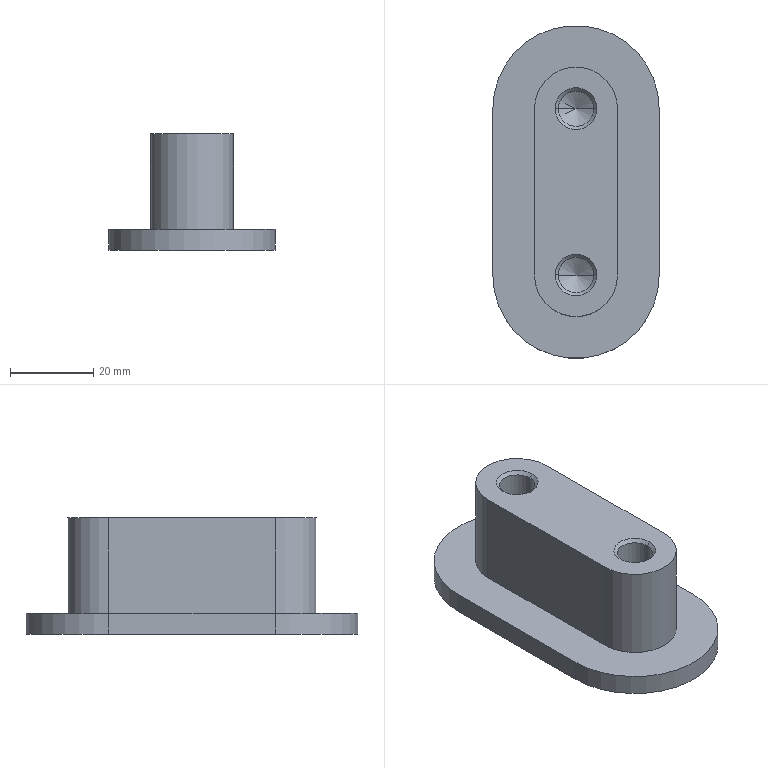Part | SolidWorks | features Extrusion 1, HoleWzd 1, ICE 1 | 1 solid | 23 faces | box 40 x 80 x 28 mm | volume 37305 mm3 | cone 8 | cylinder 8 | plane 7 | commonest cylinder face diameters 8.5 x4 20 x2 40 x2
STEP:
#1=CARTESIAN_POINT('',(-74.25,-60.,27.225));
#2=VERTEX_POINT('',#1);
#3=CARTESIAN_POINT('',(-65.75,-60.,27.225));
#4=VERTEX_POINT('',#3);
#5=CARTESIAN_POINT('',(-70.,-60.,27.225));
#6=DIRECTION('',(0.,0.,1.));
#7=DIRECTION('',(1.,0.,0.));
#8=AXIS2_PLACEMENT_3D('',#5,#6,#7);
#9=CIRCLE('',#8,4.25);
#10=EDGE_CURVE('',#2,#4,#9,.T.);
#11=ORIENTED_EDGE('',*,*,#10,.F.);
#12=CARTESIAN_POINT('',(-75.025,-60.,28.));
#13=VERTEX_POINT('',#12);
#14=CARTESIAN_POINT('',(-75.025,-60.,28.));
#15=DIRECTION('',(-0.7071,0.,0.7071));
#16=VECTOR('',#15,1000.);
#17=LINE('',#14,#16);
#18=EDGE_CURVE('',#2,#13,#17,.T.);
#19=ORIENTED_EDGE('',*,*,#18,.T.);
#20=CARTESIAN_POINT('',(-64.975,-60.,28.));
#21=VERTEX_POINT('',#20);
#22=CARTESIAN_POINT('',(-70.,-60.,28.));
#23=DIRECTION('',(0.,0.,1.));
#24=DIRECTION('',(1.,0.,0.));
#25=AXIS2_PLACEMENT_3D('',#22,#23,#24);
#26=CIRCLE('',#25,5.025);
#27=EDGE_CURVE('',#13,#21,#26,.T.);
#28=ORIENTED_EDGE('',*,*,#27,.T.);
#29=CARTESIAN_POINT('',(-64.975,-60.,28.));
#30=DIRECTION('',(0.7071,0.,0.7071));
#31=VECTOR('',#30,1000.);
#32=LINE('',#29,#31);
#33=EDGE_CURVE('',#4,#21,#32,.T.);
#34=ORIENTED_EDGE('',*,*,#33,.F.);
#35=EDGE_LOOP('',(#11,#19,#28,#34));
#36=FACE_OUTER_BOUND('',#35,.T.);
#37=CARTESIAN_POINT('',(-70.,-60.,28.));
#38=DIRECTION('',(0.,0.,1.));
#39=DIRECTION('',(1.,0.,0.));
#40=AXIS2_PLACEMENT_3D('',#37,#38,#39);
#41=CONICAL_SURFACE('',#40,5.025,0.7854);
#42=ADVANCED_FACE('',(#36),#41,.F.);
#43=CARTESIAN_POINT('',(-74.25,-60.,6.054));
#44=VERTEX_POINT('',#43);
#45=CARTESIAN_POINT('',(-65.75,-60.,6.054));
#46=VERTEX_POINT('',#45);
#47=CARTESIAN_POINT('',(-70.,-60.,6.054));
#48=DIRECTION('',(0.,0.,1.));
#49=DIRECTION('',(1.,0.,0.));
#50=AXIS2_PLACEMENT_3D('',#47,#48,#49);
#51=CIRCLE('',#50,4.25);
#52=EDGE_CURVE('',#44,#46,#51,.T.);
#53=ORIENTED_EDGE('',*,*,#52,.F.);
#54=CARTESIAN_POINT('',(-74.25,-60.,28.));
#55=DIRECTION('',(0.,0.,1.));
#56=VECTOR('',#55,1000.);
#57=LINE('',#54,#56);
#58=EDGE_CURVE('',#44,#2,#57,.T.);
#59=ORIENTED_EDGE('',*,*,#58,.T.);
#60=ORIENTED_EDGE('',*,*,#10,.T.);
#61=CARTESIAN_POINT('',(-65.75,-60.,28.));
#62=DIRECTION('',(0.,0.,1.));
#63=VECTOR('',#62,1000.);
#64=LINE('',#61,#63);
#65=EDGE_CURVE('',#46,#4,#64,.T.);
#66=ORIENTED_EDGE('',*,*,#65,.F.);
#67=EDGE_LOOP('',(#53,#59,#60,#66));
#68=FACE_OUTER_BOUND('',#67,.T.);
#69=CARTESIAN_POINT('',(-70.,-60.,28.));
#70=DIRECTION('',(0.,0.,1.));
#71=DIRECTION('',(1.,0.,0.));
#72=AXIS2_PLACEMENT_3D('',#69,#70,#71);
#73=CYLINDRICAL_SURFACE('',#72,4.25);
#74=ADVANCED_FACE('',(#68),#73,.F.);
#75=CARTESIAN_POINT('',(-70.,-60.,3.5));
#76=VERTEX_POINT('',#75);
#77=CARTESIAN_POINT('',(-65.75,-60.,6.054));
#78=DIRECTION('',(0.8572,0.,0.515));
#79=VECTOR('',#78,1000.);
#80=LINE('',#77,#79);
#81=EDGE_CURVE('',#76,#46,#80,.T.);
#82=ORIENTED_EDGE('',*,*,#81,.F.);
#83=CARTESIAN_POINT('',(-74.25,-60.,6.054));
#84=DIRECTION('',(-0.8572,0.,0.515));
#85=VECTOR('',#84,1000.);
#86=LINE('',#83,#85);
#87=EDGE_CURVE('',#76,#44,#86,.T.);
#88=ORIENTED_EDGE('',*,*,#87,.T.);
#89=ORIENTED_EDGE('',*,*,#52,.T.);
#90=EDGE_LOOP('',(#82,#88,#89));
#91=FACE_OUTER_BOUND('',#90,.T.);
#92=CARTESIAN_POINT('',(-70.,-60.,6.054));
#93=DIRECTION('',(0.,0.,1.));
#94=DIRECTION('',(1.,0.,0.));
#95=AXIS2_PLACEMENT_3D('',#92,#93,#94);
#96=CONICAL_SURFACE('',#95,4.25,1.03);
#97=ADVANCED_FACE('',(#91),#96,.F.);
#98=CARTESIAN_POINT('',(-74.25,-100.,27.225));
#99=VERTEX_POINT('',#98);
#100=CARTESIAN_POINT('',(-65.75,-100.,27.225));
#101=VERTEX_POINT('',#100);
#102=CARTESIAN_POINT('',(-70.,-100.,27.225));
#103=DIRECTION('',(0.,0.,1.));
#104=DIRECTION('',(1.,0.,0.));
#105=AXIS2_PLACEMENT_3D('',#102,#103,#104);
#106=CIRCLE('',#105,4.25);
#107=EDGE_CURVE('',#99,#101,#106,.T.);
#108=ORIENTED_EDGE('',*,*,#107,.F.);
#109=CARTESIAN_POINT('',(-75.025,-100.,28.));
#110=VERTEX_POINT('',#109);
#111=CARTESIAN_POINT('',(-75.025,-100.,28.));
#112=DIRECTION('',(-0.7071,0.,0.7071));
#113=VECTOR('',#112,1000.);
#114=LINE('',#111,#113);
#115=EDGE_CURVE('',#99,#110,#114,.T.);
#116=ORIENTED_EDGE('',*,*,#115,.T.);
#117=CARTESIAN_POINT('',(-64.975,-100.,28.));
#118=VERTEX_POINT('',#117);
#119=CARTESIAN_POINT('',(-70.,-100.,28.));
#120=DIRECTION('',(0.,0.,1.));
#121=DIRECTION('',(1.,0.,0.));
#122=AXIS2_PLACEMENT_3D('',#119,#120,#121);
#123=CIRCLE('',#122,5.025);
#124=EDGE_CURVE('',#110,#118,#123,.T.);
#125=ORIENTED_EDGE('',*,*,#124,.T.);
#126=CARTESIAN_POINT('',(-64.975,-100.,28.));
#127=DIRECTION('',(0.7071,0.,0.7071));
#128=VECTOR('',#127,1000.);
#129=LINE('',#126,#128);
#130=EDGE_CURVE('',#101,#118,#129,.T.);
#131=ORIENTED_EDGE('',*,*,#130,.F.);
#132=EDGE_LOOP('',(#108,#116,#125,#131));
#133=FACE_OUTER_BOUND('',#132,.T.);
#134=CARTESIAN_POINT('',(-70.,-100.,28.));
#135=DIRECTION('',(0.,0.,1.));
#136=DIRECTION('',(1.,0.,0.));
#137=AXIS2_PLACEMENT_3D('',#134,#135,#136);
#138=CONICAL_SURFACE('',#137,5.025,0.7854);
#139=ADVANCED_FACE('',(#133),#138,.F.);
#140=CARTESIAN_POINT('',(-74.25,-100.,6.054));
#141=VERTEX_POINT('',#140);
#142=CARTESIAN_POINT('',(-65.75,-100.,6.054));
#143=VERTEX_POINT('',#142);
#144=CARTESIAN_POINT('',(-70.,-100.,6.054));
#145=DIRECTION('',(0.,0.,1.));
#146=DIRECTION('',(1.,0.,0.));
#147=AXIS2_PLACEMENT_3D('',#144,#145,#146);
#148=CIRCLE('',#147,4.25);
#149=EDGE_CURVE('',#141,#143,#148,.T.);
#150=ORIENTED_EDGE('',*,*,#149,.F.);
#151=CARTESIAN_POINT('',(-74.25,-100.,28.));
#152=DIRECTION('',(0.,0.,1.));
#153=VECTOR('',#152,1000.);
#154=LINE('',#151,#153);
#155=EDGE_CURVE('',#141,#99,#154,.T.);
#156=ORIENTED_EDGE('',*,*,#155,.T.);
#157=ORIENTED_EDGE('',*,*,#107,.T.);
#158=CARTESIAN_POINT('',(-65.75,-100.,28.));
#159=DIRECTION('',(0.,0.,1.));
#160=VECTOR('',#159,1000.);
#161=LINE('',#158,#160);
#162=EDGE_CURVE('',#143,#101,#161,.T.);
#163=ORIENTED_EDGE('',*,*,#162,.F.);
#164=EDGE_LOOP('',(#150,#156,#157,#163));
#165=FACE_OUTER_BOUND('',#164,.T.);
#166=CARTESIAN_POINT('',(-70.,-100.,28.));
#167=DIRECTION('',(0.,0.,1.));
#168=DIRECTION('',(1.,0.,0.));
#169=AXIS2_PLACEMENT_3D('',#166,#167,#168);
#170=CYLINDRICAL_SURFACE('',#169,4.25);
#171=ADVANCED_FACE('',(#165),#170,.F.);
#172=CARTESIAN_POINT('',(-70.,-100.,3.5));
#173=VERTEX_POINT('',#172);
#174=CARTESIAN_POINT('',(-65.75,-100.,6.054));
#175=DIRECTION('',(0.8572,0.,0.515));
#176=VECTOR('',#175,1000.);
#177=LINE('',#174,#176);
#178=EDGE_CURVE('',#173,#143,#177,.T.);
#179=ORIENTED_EDGE('',*,*,#178,.F.);
#180=CARTESIAN_POINT('',(-74.25,-100.,6.054));
#181=DIRECTION('',(-0.8572,0.,0.515));
#182=VECTOR('',#181,1000.);
#183=LINE('',#180,#182);
#184=EDGE_CURVE('',#173,#141,#183,.T.);
#185=ORIENTED_EDGE('',*,*,#184,.T.);
#186=ORIENTED_EDGE('',*,*,#149,.T.);
#187=EDGE_LOOP('',(#179,#185,#186));
#188=FACE_OUTER_BOUND('',#187,.T.);
#189=CARTESIAN_POINT('',(-70.,-100.,6.054));
#190=DIRECTION('',(0.,0.,1.));
#191=DIRECTION('',(1.,0.,0.));
#192=AXIS2_PLACEMENT_3D('',#189,#190,#191);
#193=CONICAL_SURFACE('',#192,4.25,1.03);
#194=ADVANCED_FACE('',(#188),#193,.F.);
#195=CARTESIAN_POINT('',(-60.,-60.,28.));
#196=VERTEX_POINT('',#195);
#197=CARTESIAN_POINT('',(-60.,-60.,5.));
#198=VERTEX_POINT('',#197);
#199=CARTESIAN_POINT('',(-60.,-60.,28.));
#200=DIRECTION('',(0.,0.,-1.));
#201=VECTOR('',#200,1000.);
#202=LINE('',#199,#201);
#203=EDGE_CURVE('',#196,#198,#202,.T.);
#204=ORIENTED_EDGE('',*,*,#203,.T.);
#205=CARTESIAN_POINT('',(-80.,-60.,5.));
#206=VERTEX_POINT('',#205);
#207=CARTESIAN_POINT('',(-70.,-60.,5.));
#208=DIRECTION('',(0.,0.,1.));
#209=DIRECTION('',(1.,0.,0.));
#210=AXIS2_PLACEMENT_3D('',#207,#208,#209);
#211=CIRCLE('',#210,10.);
#212=EDGE_CURVE('',#198,#206,#211,.T.);
#213=ORIENTED_EDGE('',*,*,#212,.T.);
#214=CARTESIAN_POINT('',(-80.,-60.,28.));
#215=VERTEX_POINT('',#214);
#216=CARTESIAN_POINT('',(-80.,-60.,28.));
#217=DIRECTION('',(0.,0.,-1.));
#218=VECTOR('',#217,1000.);
#219=LINE('',#216,#218);
#220=EDGE_CURVE('',#215,#206,#219,.T.);
#221=ORIENTED_EDGE('',*,*,#220,.F.);
#222=CARTESIAN_POINT('',(-70.,-60.,28.));
#223=DIRECTION('',(0.,0.,1.));
#224=DIRECTION('',(1.,0.,0.));
#225=AXIS2_PLACEMENT_3D('',#222,#223,#224);
#226=CIRCLE('',#225,10.);
#227=EDGE_CURVE('',#196,#215,#226,.T.);
#228=ORIENTED_EDGE('',*,*,#227,.F.);
#229=EDGE_LOOP('',(#204,#213,#221,#228));
#230=FACE_OUTER_BOUND('',#229,.T.);
#231=CARTESIAN_POINT('',(-70.,-60.,28.));
#232=DIRECTION('',(0.,0.,-1.));
#233=DIRECTION('',(-1.,0.,0.));
#234=AXIS2_PLACEMENT_3D('',#231,#232,#233);
#235=CYLINDRICAL_SURFACE('',#234,10.);
#236=ADVANCED_FACE('',(#230),#235,.T.);
#237=ORIENTED_EDGE('',*,*,#220,.T.);
#238=CARTESIAN_POINT('',(-80.,-100.,5.));
#239=VERTEX_POINT('',#238);
#240=CARTESIAN_POINT('',(-80.,-60.,5.));
#241=DIRECTION('',(0.,-1.,0.));
#242=VECTOR('',#241,1000.);
#243=LINE('',#240,#242);
#244=EDGE_CURVE('',#206,#239,#243,.T.);
#245=ORIENTED_EDGE('',*,*,#244,.T.);
#246=CARTESIAN_POINT('',(-80.,-100.,28.));
#247=VERTEX_POINT('',#246);
#248=CARTESIAN_POINT('',(-80.,-100.,28.));
#249=DIRECTION('',(0.,0.,-1.));
#250=VECTOR('',#249,1000.);
#251=LINE('',#248,#250);
#252=EDGE_CURVE('',#247,#239,#251,.T.);
#253=ORIENTED_EDGE('',*,*,#252,.F.);
#254=CARTESIAN_POINT('',(-80.,-60.,28.));
#255=DIRECTION('',(0.,-1.,0.));
#256=VECTOR('',#255,1000.);
#257=LINE('',#254,#256);
#258=EDGE_CURVE('',#215,#247,#257,.T.);
#259=ORIENTED_EDGE('',*,*,#258,.F.);
#260=EDGE_LOOP('',(#237,#245,#253,#259));
#261=FACE_OUTER_BOUND('',#260,.T.);
#262=CARTESIAN_POINT('',(-80.,-60.,28.));
#263=DIRECTION('',(1.,0.,0.));
#264=DIRECTION('',(0.,0.,-1.));
#265=AXIS2_PLACEMENT_3D('',#262,#263,#264);
#266=PLANE('',#265);
#267=ADVANCED_FACE('',(#261),#266,.F.);
#268=ORIENTED_EDGE('',*,*,#252,.T.);
#269=CARTESIAN_POINT('',(-60.,-100.,5.));
#270=VERTEX_POINT('',#269);
#271=CARTESIAN_POINT('',(-70.,-100.,5.));
#272=DIRECTION('',(0.,0.,1.));
#273=DIRECTION('',(1.,0.,0.));
#274=AXIS2_PLACEMENT_3D('',#271,#272,#273);
#275=CIRCLE('',#274,10.);
#276=EDGE_CURVE('',#239,#270,#275,.T.);
#277=ORIENTED_EDGE('',*,*,#276,.T.);
#278=CARTESIAN_POINT('',(-60.,-100.,28.));
#279=VERTEX_POINT('',#278);
#280=CARTESIAN_POINT('',(-60.,-100.,28.));
#281=DIRECTION('',(0.,0.,-1.));
#282=VECTOR('',#281,1000.);
#283=LINE('',#280,#282);
#284=EDGE_CURVE('',#279,#270,#283,.T.);
#285=ORIENTED_EDGE('',*,*,#284,.F.);
#286=CARTESIAN_POINT('',(-70.,-100.,28.));
#287=DIRECTION('',(0.,0.,1.));
#288=DIRECTION('',(1.,0.,0.));
#289=AXIS2_PLACEMENT_3D('',#286,#287,#288);
#290=CIRCLE('',#289,10.);
#291=EDGE_CURVE('',#247,#279,#290,.T.);
#292=ORIENTED_EDGE('',*,*,#291,.F.);
#293=EDGE_LOOP('',(#268,#277,#285,#292));
#294=FACE_OUTER_BOUND('',#293,.T.);
#295=CARTESIAN_POINT('',(-70.,-100.,28.));
#296=DIRECTION('',(0.,0.,-1.));
#297=DIRECTION('',(-1.,0.,0.));
#298=AXIS2_PLACEMENT_3D('',#295,#296,#297);
#299=CYLINDRICAL_SURFACE('',#298,10.);
#300=ADVANCED_FACE('',(#294),#299,.T.);
#301=ORIENTED_EDGE('',*,*,#284,.T.);
#302=CARTESIAN_POINT('',(-60.,-60.,5.));
#303=DIRECTION('',(0.,1.,0.));
#304=VECTOR('',#303,1000.);
#305=LINE('',#302,#304);
#306=EDGE_CURVE('',#270,#198,#305,.T.);
#307=ORIENTED_EDGE('',*,*,#306,.T.);
#308=ORIENTED_EDGE('',*,*,#203,.F.);
#309=CARTESIAN_POINT('',(-60.,-60.,28.));
#310=DIRECTION('',(0.,1.,0.));
#311=VECTOR('',#310,1000.);
#312=LINE('',#309,#311);
#313=EDGE_CURVE('',#279,#196,#312,.T.);
#314=ORIENTED_EDGE('',*,*,#313,.F.);
#315=EDGE_LOOP('',(#301,#307,#308,#314));
#316=FACE_OUTER_BOUND('',#315,.T.);
#317=CARTESIAN_POINT('',(-60.,-60.,28.));
#318=DIRECTION('',(-1.,0.,0.));
#319=DIRECTION('',(0.,0.,1.));
#320=AXIS2_PLACEMENT_3D('',#317,#318,#319);
#321=PLANE('',#320);
#322=ADVANCED_FACE('',(#316),#321,.F.);
#323=CARTESIAN_POINT('',(-70.,-60.,28.));
#324=DIRECTION('',(0.,0.,1.));
#325=DIRECTION('',(1.,0.,0.));
#326=AXIS2_PLACEMENT_3D('',#323,#324,#325);
#327=CIRCLE('',#326,5.025);
#328=EDGE_CURVE('',#21,#13,#327,.T.);
#329=ORIENTED_EDGE('',*,*,#328,.F.);
#330=ORIENTED_EDGE('',*,*,#27,.F.);
#331=EDGE_LOOP('',(#329,#330));
#332=FACE_BOUND('',#331,.T.);
#333=CARTESIAN_POINT('',(-70.,-100.,28.));
#334=DIRECTION('',(0.,0.,1.));
#335=DIRECTION('',(1.,0.,0.));
#336=AXIS2_PLACEMENT_3D('',#333,#334,#335);
#337=CIRCLE('',#336,5.025);
#338=EDGE_CURVE('',#118,#110,#337,.T.);
#339=ORIENTED_EDGE('',*,*,#338,.F.);
#340=ORIENTED_EDGE('',*,*,#124,.F.);
#341=EDGE_LOOP('',(#339,#340));
#342=FACE_BOUND('',#341,.T.);
#343=ORIENTED_EDGE('',*,*,#227,.T.);
#344=ORIENTED_EDGE('',*,*,#258,.T.);
#345=ORIENTED_EDGE('',*,*,#291,.T.);
#346=ORIENTED_EDGE('',*,*,#313,.T.);
#347=EDGE_LOOP('',(#343,#344,#345,#346));
#348=FACE_OUTER_BOUND('',#347,.T.);
#349=CARTESIAN_POINT('',(-70.,-60.,28.));
#350=DIRECTION('',(0.,0.,1.));
#351=DIRECTION('',(1.,0.,0.));
#352=AXIS2_PLACEMENT_3D('',#349,#350,#351);
#353=PLANE('',#352);
#354=ADVANCED_FACE('',(#332,#342,#348),#353,.T.);
#355=CARTESIAN_POINT('',(-50.,-60.,5.));
#356=VERTEX_POINT('',#355);
#357=CARTESIAN_POINT('',(-90.,-60.,5.));
#358=VERTEX_POINT('',#357);
#359=CARTESIAN_POINT('',(-70.,-60.,5.));
#360=DIRECTION('',(0.,0.,1.));
#361=DIRECTION('',(1.,0.,0.));
#362=AXIS2_PLACEMENT_3D('',#359,#360,#361);
#363=CIRCLE('',#362,20.);
#364=EDGE_CURVE('',#356,#358,#363,.T.);
#365=ORIENTED_EDGE('',*,*,#364,.T.);
#366=CARTESIAN_POINT('',(-90.,-100.,5.));
#367=VERTEX_POINT('',#366);
#368=CARTESIAN_POINT('',(-90.,-60.,5.));
#369=DIRECTION('',(0.,-1.,0.));
#370=VECTOR('',#369,1000.);
#371=LINE('',#368,#370);
#372=EDGE_CURVE('',#358,#367,#371,.T.);
#373=ORIENTED_EDGE('',*,*,#372,.T.);
#374=CARTESIAN_POINT('',(-50.,-100.,5.));
#375=VERTEX_POINT('',#374);
#376=CARTESIAN_POINT('',(-70.,-100.,5.));
#377=DIRECTION('',(0.,0.,1.));
#378=DIRECTION('',(1.,0.,0.));
#379=AXIS2_PLACEMENT_3D('',#376,#377,#378);
#380=CIRCLE('',#379,20.);
#381=EDGE_CURVE('',#367,#375,#380,.T.);
#382=ORIENTED_EDGE('',*,*,#381,.T.);
#383=CARTESIAN_POINT('',(-50.,-100.,5.));
#384=DIRECTION('',(0.,1.,0.));
#385=VECTOR('',#384,1000.);
#386=LINE('',#383,#385);
#387=EDGE_CURVE('',#375,#356,#386,.T.);
#388=ORIENTED_EDGE('',*,*,#387,.T.);
#389=EDGE_LOOP('',(#365,#373,#382,#388));
#390=FACE_OUTER_BOUND('',#389,.T.);
#391=ORIENTED_EDGE('',*,*,#212,.F.);
#392=ORIENTED_EDGE('',*,*,#306,.F.);
#393=ORIENTED_EDGE('',*,*,#276,.F.);
#394=ORIENTED_EDGE('',*,*,#244,.F.);
#395=EDGE_LOOP('',(#391,#392,#393,#394));
#396=FACE_BOUND('',#395,.T.);
#397=CARTESIAN_POINT('',(-70.,-60.,5.));
#398=DIRECTION('',(0.,0.,1.));
#399=DIRECTION('',(1.,0.,0.));
#400=AXIS2_PLACEMENT_3D('',#397,#398,#399);
#401=PLANE('',#400);
#402=ADVANCED_FACE('',(#390,#396),#401,.T.);
#403=CARTESIAN_POINT('',(-50.,-60.,0.));
#404=VERTEX_POINT('',#403);
#405=CARTESIAN_POINT('',(-90.,-60.,0.));
#406=VERTEX_POINT('',#405);
#407=CARTESIAN_POINT('',(-70.,-60.,0.));
#408=DIRECTION('',(0.,0.,1.));
#409=DIRECTION('',(1.,0.,0.));
#410=AXIS2_PLACEMENT_3D('',#407,#408,#409);
#411=CIRCLE('',#410,20.);
#412=EDGE_CURVE('',#404,#406,#411,.T.);
#413=ORIENTED_EDGE('',*,*,#412,.T.);
#414=CARTESIAN_POINT('',(-90.,-60.,5.));
#415=DIRECTION('',(0.,0.,-1.));
#416=VECTOR('',#415,1000.);
#417=LINE('',#414,#416);
#418=EDGE_CURVE('',#358,#406,#417,.T.);
#419=ORIENTED_EDGE('',*,*,#418,.F.);
#420=ORIENTED_EDGE('',*,*,#364,.F.);
#421=CARTESIAN_POINT('',(-50.,-60.,5.));
#422=DIRECTION('',(0.,0.,-1.));
#423=VECTOR('',#422,1000.);
#424=LINE('',#421,#423);
#425=EDGE_CURVE('',#356,#404,#424,.T.);
#426=ORIENTED_EDGE('',*,*,#425,.T.);
#427=EDGE_LOOP('',(#413,#419,#420,#426));
#428=FACE_OUTER_BOUND('',#427,.T.);
#429=CARTESIAN_POINT('',(-70.,-60.,5.));
#430=DIRECTION('',(0.,0.,-1.));
#431=DIRECTION('',(-1.,0.,0.));
#432=AXIS2_PLACEMENT_3D('',#429,#430,#431);
#433=CYLINDRICAL_SURFACE('',#432,20.);
#434=ADVANCED_FACE('',(#428),#433,.T.);
#435=CARTESIAN_POINT('',(-90.,-100.,0.));
#436=VERTEX_POINT('',#435);
#437=CARTESIAN_POINT('',(-90.,-60.,0.));
#438=DIRECTION('',(0.,-1.,0.));
#439=VECTOR('',#438,1000.);
#440=LINE('',#437,#439);
#441=EDGE_CURVE('',#406,#436,#440,.T.);
#442=ORIENTED_EDGE('',*,*,#441,.T.);
#443=CARTESIAN_POINT('',(-90.,-100.,5.));
#444=DIRECTION('',(0.,0.,-1.));
#445=VECTOR('',#444,1000.);
#446=LINE('',#443,#445);
#447=EDGE_CURVE('',#367,#436,#446,.T.);
#448=ORIENTED_EDGE('',*,*,#447,.F.);
#449=ORIENTED_EDGE('',*,*,#372,.F.);
#450=ORIENTED_EDGE('',*,*,#418,.T.);
#451=EDGE_LOOP('',(#442,#448,#449,#450));
#452=FACE_OUTER_BOUND('',#451,.T.);
#453=CARTESIAN_POINT('',(-90.,-60.,5.));
#454=DIRECTION('',(1.,0.,0.));
#455=DIRECTION('',(0.,1.,0.));
#456=AXIS2_PLACEMENT_3D('',#453,#454,#455);
#457=PLANE('',#456);
#458=ADVANCED_FACE('',(#452),#457,.F.);
#459=CARTESIAN_POINT('',(-50.,-100.,0.));
#460=VERTEX_POINT('',#459);
#461=CARTESIAN_POINT('',(-70.,-100.,0.));
#462=DIRECTION('',(0.,0.,1.));
#463=DIRECTION('',(1.,0.,0.));
#464=AXIS2_PLACEMENT_3D('',#461,#462,#463);
#465=CIRCLE('',#464,20.);
#466=EDGE_CURVE('',#436,#460,#465,.T.);
#467=ORIENTED_EDGE('',*,*,#466,.T.);
#468=CARTESIAN_POINT('',(-50.,-100.,5.));
#469=DIRECTION('',(0.,0.,-1.));
#470=VECTOR('',#469,1000.);
#471=LINE('',#468,#470);
#472=EDGE_CURVE('',#375,#460,#471,.T.);
#473=ORIENTED_EDGE('',*,*,#472,.F.);
#474=ORIENTED_EDGE('',*,*,#381,.F.);
#475=ORIENTED_EDGE('',*,*,#447,.T.);
#476=EDGE_LOOP('',(#467,#473,#474,#475));
#477=FACE_OUTER_BOUND('',#476,.T.);
#478=CARTESIAN_POINT('',(-70.,-100.,5.));
#479=DIRECTION('',(0.,0.,-1.));
#480=DIRECTION('',(-1.,0.,0.));
#481=AXIS2_PLACEMENT_3D('',#478,#479,#480);
#482=CYLINDRICAL_SURFACE('',#481,20.);
#483=ADVANCED_FACE('',(#477),#482,.T.);
#484=CARTESIAN_POINT('',(-50.,-100.,0.));
#485=DIRECTION('',(0.,1.,0.));
#486=VECTOR('',#485,1000.);
#487=LINE('',#484,#486);
#488=EDGE_CURVE('',#460,#404,#487,.T.);
#489=ORIENTED_EDGE('',*,*,#488,.T.);
#490=ORIENTED_EDGE('',*,*,#425,.F.);
#491=ORIENTED_EDGE('',*,*,#387,.F.);
#492=ORIENTED_EDGE('',*,*,#472,.T.);
#493=EDGE_LOOP('',(#489,#490,#491,#492));
#494=FACE_OUTER_BOUND('',#493,.T.);
#495=CARTESIAN_POINT('',(-50.,-100.,5.));
#496=DIRECTION('',(-1.,0.,0.));
#497=DIRECTION('',(0.,-1.,0.));
#498=AXIS2_PLACEMENT_3D('',#495,#496,#497);
#499=PLANE('',#498);
#500=ADVANCED_FACE('',(#494),#499,.F.);
#501=ORIENTED_EDGE('',*,*,#412,.F.);
#502=ORIENTED_EDGE('',*,*,#488,.F.);
#503=ORIENTED_EDGE('',*,*,#466,.F.);
#504=ORIENTED_EDGE('',*,*,#441,.F.);
#505=EDGE_LOOP('',(#501,#502,#503,#504));
#506=FACE_OUTER_BOUND('',#505,.T.);
#507=CARTESIAN_POINT('',(-70.,-60.,0.));
#508=DIRECTION('',(0.,0.,1.));
#509=DIRECTION('',(1.,0.,0.));
#510=AXIS2_PLACEMENT_3D('',#507,#508,#509);
#511=PLANE('',#510);
#512=ADVANCED_FACE('',(#506),#511,.F.);
#513=ORIENTED_EDGE('',*,*,#184,.F.);
#514=ORIENTED_EDGE('',*,*,#178,.T.);
#515=CARTESIAN_POINT('',(-70.,-100.,6.054));
#516=DIRECTION('',(0.,0.,1.));
#517=DIRECTION('',(1.,0.,0.));
#518=AXIS2_PLACEMENT_3D('',#515,#516,#517);
#519=CIRCLE('',#518,4.25);
#520=EDGE_CURVE('',#143,#141,#519,.T.);
#521=ORIENTED_EDGE('',*,*,#520,.T.);
#522=EDGE_LOOP('',(#513,#514,#521));
#523=FACE_OUTER_BOUND('',#522,.T.);
#524=CARTESIAN_POINT('',(-70.,-100.,6.054));
#525=DIRECTION('',(0.,0.,1.));
#526=DIRECTION('',(1.,0.,0.));
#527=AXIS2_PLACEMENT_3D('',#524,#525,#526);
#528=CONICAL_SURFACE('',#527,4.25,1.03);
#529=ADVANCED_FACE('',(#523),#528,.F.);
#530=ORIENTED_EDGE('',*,*,#155,.F.);
#531=ORIENTED_EDGE('',*,*,#520,.F.);
#532=ORIENTED_EDGE('',*,*,#162,.T.);
#533=CARTESIAN_POINT('',(-70.,-100.,27.225));
#534=DIRECTION('',(0.,0.,1.));
#535=DIRECTION('',(1.,0.,0.));
#536=AXIS2_PLACEMENT_3D('',#533,#534,#535);
#537=CIRCLE('',#536,4.25);
#538=EDGE_CURVE('',#101,#99,#537,.T.);
#539=ORIENTED_EDGE('',*,*,#538,.T.);
#540=EDGE_LOOP('',(#530,#531,#532,#539));
#541=FACE_OUTER_BOUND('',#540,.T.);
#542=CARTESIAN_POINT('',(-70.,-100.,28.));
#543=DIRECTION('',(0.,0.,1.));
#544=DIRECTION('',(1.,0.,0.));
#545=AXIS2_PLACEMENT_3D('',#542,#543,#544);
#546=CYLINDRICAL_SURFACE('',#545,4.25);
#547=ADVANCED_FACE('',(#541),#546,.F.);
#548=ORIENTED_EDGE('',*,*,#115,.F.);
#549=ORIENTED_EDGE('',*,*,#538,.F.);
#550=ORIENTED_EDGE('',*,*,#130,.T.);
#551=ORIENTED_EDGE('',*,*,#338,.T.);
#552=EDGE_LOOP('',(#548,#549,#550,#551));
#553=FACE_OUTER_BOUND('',#552,.T.);
#554=CARTESIAN_POINT('',(-70.,-100.,28.));
#555=DIRECTION('',(0.,0.,1.));
#556=DIRECTION('',(1.,0.,0.));
#557=AXIS2_PLACEMENT_3D('',#554,#555,#556);
#558=CONICAL_SURFACE('',#557,5.025,0.7854);
#559=ADVANCED_FACE('',(#553),#558,.F.);
#560=ORIENTED_EDGE('',*,*,#87,.F.);
#561=ORIENTED_EDGE('',*,*,#81,.T.);
#562=CARTESIAN_POINT('',(-70.,-60.,6.054));
#563=DIRECTION('',(0.,0.,1.));
#564=DIRECTION('',(1.,0.,0.));
#565=AXIS2_PLACEMENT_3D('',#562,#563,#564);
#566=CIRCLE('',#565,4.25);
#567=EDGE_CURVE('',#46,#44,#566,.T.);
#568=ORIENTED_EDGE('',*,*,#567,.T.);
#569=EDGE_LOOP('',(#560,#561,#568));
#570=FACE_OUTER_BOUND('',#569,.T.);
#571=CARTESIAN_POINT('',(-70.,-60.,6.054));
#572=DIRECTION('',(0.,0.,1.));
#573=DIRECTION('',(1.,0.,0.));
#574=AXIS2_PLACEMENT_3D('',#571,#572,#573);
#575=CONICAL_SURFACE('',#574,4.25,1.03);
#576=ADVANCED_FACE('',(#570),#575,.F.);
#577=ORIENTED_EDGE('',*,*,#58,.F.);
#578=ORIENTED_EDGE('',*,*,#567,.F.);
#579=ORIENTED_EDGE('',*,*,#65,.T.);
#580=CARTESIAN_POINT('',(-70.,-60.,27.225));
#581=DIRECTION('',(0.,0.,1.));
#582=DIRECTION('',(1.,0.,0.));
#583=AXIS2_PLACEMENT_3D('',#580,#581,#582);
#584=CIRCLE('',#583,4.25);
#585=EDGE_CURVE('',#4,#2,#584,.T.);
#586=ORIENTED_EDGE('',*,*,#585,.T.);
#587=EDGE_LOOP('',(#577,#578,#579,#586));
#588=FACE_OUTER_BOUND('',#587,.T.);
#589=CARTESIAN_POINT('',(-70.,-60.,28.));
#590=DIRECTION('',(0.,0.,1.));
#591=DIRECTION('',(1.,0.,0.));
#592=AXIS2_PLACEMENT_3D('',#589,#590,#591);
#593=CYLINDRICAL_SURFACE('',#592,4.25);
#594=ADVANCED_FACE('',(#588),#593,.F.);
#595=ORIENTED_EDGE('',*,*,#18,.F.);
#596=ORIENTED_EDGE('',*,*,#585,.F.);
#597=ORIENTED_EDGE('',*,*,#33,.T.);
#598=ORIENTED_EDGE('',*,*,#328,.T.);
#599=EDGE_LOOP('',(#595,#596,#597,#598));
#600=FACE_OUTER_BOUND('',#599,.T.);
#601=CARTESIAN_POINT('',(-70.,-60.,28.));
#602=DIRECTION('',(0.,0.,1.));
#603=DIRECTION('',(1.,0.,0.));
#604=AXIS2_PLACEMENT_3D('',#601,#602,#603);
#605=CONICAL_SURFACE('',#604,5.025,0.7854);
#606=ADVANCED_FACE('',(#600),#605,.F.);
#607=CLOSED_SHELL('',(#42,#74,#97,#139,#171,#194,#236,#267,#300,#322,#354,#402,#434,#458,#483,#500,#512,#529,#547,#559,#576,#594,#606));
#608=MANIFOLD_SOLID_BREP('',#607);
#609=CARTESIAN_POINT('',(0.,0.,0.));
#610=DIRECTION('',(0.,0.,1.));
#611=DIRECTION('',(1.,0.,0.));
#612=AXIS2_PLACEMENT_3D('',#609,#610,#611);
#613=(LENGTH_UNIT()NAMED_UNIT(*)SI_UNIT(.MILLI.,.METRE.));
#614=UNCERTAINTY_MEASURE_WITH_UNIT(LENGTH_MEASURE(0.00001),#613,'','');
#615=(NAMED_UNIT(*)PLANE_ANGLE_UNIT()SI_UNIT($,.RADIAN.));
#616=(NAMED_UNIT(*)SI_UNIT($,.STERADIAN.)SOLID_ANGLE_UNIT());
#617=(GEOMETRIC_REPRESENTATION_CONTEXT(3)GLOBAL_UNCERTAINTY_ASSIGNED_CONTEXT((#614))GLOBAL_UNIT_ASSIGNED_CONTEXT((#613,#615,#616))REPRESENTATION_CONTEXT('',''));
#618=ADVANCED_BREP_SHAPE_REPRESENTATION('',(#608,#612),#617);